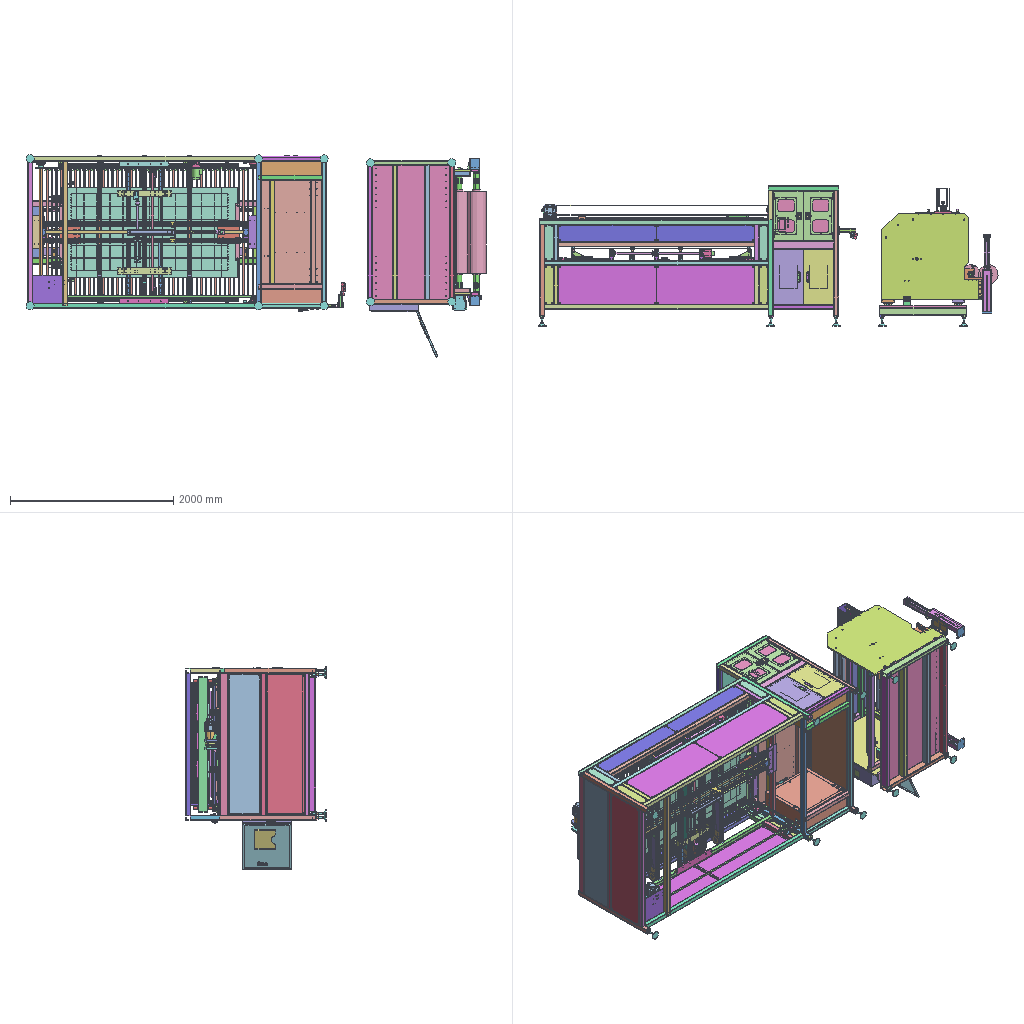Assembly | SolidWorks | 447 different items | 1108 placed | box 5632 x 1720 x 2483 mm
Parts list (item | name | quantity | parent item | size | volume | features), first 280 of 447 items:
1 | (subassembly) | x2 | in 11 | 1620 x 240 x 240 mm | 47963856 mm3 | -
2 | (subassembly) | x4 | in 1 | 35 x 74 x 74 mm | 78913 mm3 | -
3 | (subassembly) | x1 | in 11 | 170 x 962 x 160 mm | 3347225 mm3 | -
4 | (subassembly) | x1 | in 11 | 170 x 962 x 160 mm | 3347226 mm3 | -
5 | (subassembly) | x1 | in 11 | 355 x 191 x 196 mm | 4077245 mm3 | -
6 | (subassembly) | x1 | in 5 | 196 x 150 x 150 mm | 792513 mm3 | features CompositeCurve 1
7 | (subassembly) | x1 | in 11 | - | 4434874 mm3 | -
8 | (subassembly) | x2 | in 11 | 108.5 x 1345 x 60 mm | 327193 mm3 | -
9 | (subassembly) | x1 | in 11 | 130 x 80 x 80 mm | 636586 mm3 | -
10 | (subassembly) | x2 | in 58 | 70 x 30.5 x 82 mm | 109676 mm3 | -
11 | (subassembly) | x1 | - | - | 235835811 mm3 | features CompositeCurve 4
12 | (subassembly) | x1 | - | 310 x 227.812 x 145.36 mm | 532753 mm3 | -
13 | (subassembly) | x1 | - | - | - | features CompositeCurve 4, ReferencePattern 3, LocalLPattern 1
14 | (subassembly) | x1 | in 13 | - | 137447559 mm3 | features CompositeCurve 5, ReferencePattern 4, LocalLPattern 3
15 | (subassembly) | x1 | in 14 | 3660 x 1605 x 1860 mm | 102474394 mm3 | features ReferencePattern 16, LocalLPattern 3
16 | (subassembly) | x3 | in 14 | 369.222 x 614 x 49.278 mm | 1337700 mm3 | features ReferencePattern 3, CompositeCurve 1, LocalLPattern 1
17 | (subassembly) | x1 | in 14 | 369.222 x 614 x 123.704 mm | 919283 mm3 | features ReferencePattern 3, CompositeCurve 1, LocalLPattern 1
18 | (subassembly) | x1 | in 14 | 736 x 670 x 303 mm | 3762894 mm3 | features AEMSimFeature 1, MirrorCompFeat 1, ReferencePattern 1
19 | (subassembly) | x2 | in 18, 20 | 366 x 670 x 34.5 mm | 525345 mm3 | -
20 | (subassembly) | x1 | in 14 | 736 x 670 x 303 mm | 3679294 mm3 | features AEMSimFeature 1, MirrorCompFeat 1, ReferencePattern 1
21 | (subassembly) | x1 | in 13 | - | 15158359 mm3 | features ReferencePattern 23, LocalLPattern 6, CompositeCurve 3
22 | (subassembly) | x1 | in 11 | - | 105601898 mm3 | features CompositeCurve 2
23 | (subassembly) | x3 | in 21 | 45 x 115 x 115 mm | 326857 mm3 | -
24 | (subassembly) | x4 | in 21 | 45 x 50 x 50 mm | 36645 mm3 | features ReferencePattern 2, AEMSimFeature 1, MirrorCompFeat 1
25 | (subassembly) | x1 | in 13 | - | 38951088 mm3 | features ReferencePattern 10, LocalLPattern 2, AEMSimFeature 1, CompositeCurve 1
26 | (subassembly) | x1 | in 25 | 250 x 70 x 113 mm | 559339 mm3 | features AEMSimFeature 1, CompositeCurve 1
27 | (subassembly) | x1 | in 25 | 250 x 70 x 102 mm | 529348 mm3 | features AEMSimFeature 1
28 | (subassembly) | x2 | in 25 | 700 x 260 x 150.5 mm | 1942700 mm3 | features AEMSimFeature 1
29 | (subassembly) | x4 | in 28 | 40 x 40 x 85 mm | 60993 mm3 | -
30 | (subassembly) | x2 | in 25 | 666 x 259.2 x 380 mm | 1864950 mm3 | features CompositeCurve 1
31 | (subassembly) | x4 | in 30 | 58 x 169.2 x 52 mm | 267597 mm3 | -
32 | (subassembly) | x1 | in 25 | 70 x 80 x 68 mm | 209105 mm3 | features AEMSimFeature 1
33 | (subassembly) | x1 | in 22 | 837.099 x 600 x 769.432 mm | 2776594 mm3 | -
34 | (subassembly) | x1 | in 25 | 70 x 80 x 123.5 mm | 332483 mm3 | features AEMSimFeature 1
35 | (subassembly) | x1 | in 25 | 100 x 127.228 x 104 mm | 594997 mm3 | features AEMSimFeature 1, CompositeCurve 1
36 | (subassembly) | x1 | in 25 | 88 x 104 x 125 mm | 527898 mm3 | features AEMSimFeature 1
37 | (subassembly) | x1 | in 25 | 70 x 80 x 127.4 mm | 342161 mm3 | features AEMSimFeature 1
38 | (subassembly) | x1 | in 13 | - | 15629653 mm3 | features ReferencePattern 12, LocalLPattern 4, CompositeCurve 3
39 | (subassembly) | x1 | in 38 | 166.5 x 115 x 180 mm | 1052923 mm3 | features CompositeCurve 2
40 | (subassembly) | x1 | in 38 | 180 x 185 x 472 mm | 5233000 mm3 | features CompositeCurve 1
41 | (subassembly) | x1 | in 13 | - | 13271643 mm3 | features ReferencePattern 44, CompositeCurve 1, LocalLPattern 1
42 | (subassembly) | x6 | in 41 | 150 x 115.004 x 82 mm | 375409 mm3 | -
43 | (subassembly) | x1 | in 13 | 200 x 235 x 205 mm | 2926314 mm3 | -
44 | (subassembly) | x1 | in 33 | 600 x 600 x 208.5 mm | 1307519 mm3 | features LocalLPattern 1, ReferencePattern 1
45 | (subassembly) | x1 | in 13 | - | 14966347 mm3 | features ReferencePattern 9, LocalLPattern 3, CompositeCurve 2
46 | (subassembly) | x1 | in 45 | 182.5 x 100 x 174 mm | 654284 mm3 | features CompositeCurve 1
47 | (subassembly) | x1 | in 45 | 140 x 100 x 98 mm | 529951 mm3 | -
48 | (subassembly) | x1 | in 13 | - | 25836003 mm3 | -
49 | (subassembly) | x1 | in 48 | 210 x 1644 x 211.13 mm | 12241603 mm3 | features ReferencePattern 8, CompositeCurve 5, MirrorCompFeat 2
50 | (subassembly) | x1 | in 13 | - | 40703347 mm3 | features ReferencePattern 12, CompositeCurve 4, LocalLPattern 1
51 | (subassembly) | x1 | in 13 | 120 x 60 x 1710 mm | 2689604 mm3 | -
52 | (subassembly) | x1 | in 13 | 200 x 393 x 205 mm | 2855185 mm3 | -
53 | (subassembly) | x1 | in 13 | 2200 x 69.8 x 40 mm | 1056150 mm3 | features LocalLPattern 1, ReferencePattern 1
54 | (subassembly) | x8 | in 53, 57 | 22 x 67.2 x 26 mm | 3815 mm3 | features CompositeCurve 1
55 | (subassembly) | x1 | in 33 | 616.798 x 600 x 38.851 mm | 818238 mm3 | features LocalLPattern 1, ReferencePattern 1
56 | (subassembly) | x1 | in 13 | 407 x 121.237 x 1540 mm | 1039556 mm3 | -
57 | (subassembly) | x1 | in 13 | 2550 x 69.8 x 40 mm | 1229984 mm3 | features ReferencePattern 4, LocalLPattern 3
58 | (subassembly) | x2 | in 38 | 70 x 36 x 2500 mm | 1159960 mm3 | -
59 | (subassembly) | x10 | in 14, 22 | 100 x 168 x 100 mm | 203104 mm3 | -
60 | (subassembly) | x8 | in 14 | 35 x 42 x 37 mm | 5177 mm3 | -
61 | (subassembly) | x1 | in 21 | 137.5 x 90 x 275 mm | 2048853 mm3 | -
62 | (subassembly) | x1 | in 25 | 75 x 75 x 1095 mm | 1179276 mm3 | -
63 | (subassembly) | x1 | in 25 | 369 x 75 x 75 mm | 826991 mm3 | -
64 | (subassembly) | x1 | in 25 | 1100 x 2150 x 6.1 mm | 13387915 mm3 | features ReferencePattern 5, AEMSimFeature 1, LocalLPattern 1
65 | (subassembly) | x4 | in 31 | 58 x 140.2 x 52 mm | 211701 mm3 | -
66 | (subassembly) | x4 | in 11 | 60 x 60 x 1489 mm | 2237617 mm3 | -
67 | (subassembly) | x5 | in 38 | 57 x 23 x 16 mm | 13388 mm3 | -
68 | (subassembly) | x3 | in 38 | 254 x 83 x 36 mm | 461656 mm3 | -
69 | (subassembly) | x2 | in 41 | 108 x 108 x 40.2 mm | 171689 mm3 | -
70 | (subassembly) | x1 | in 45 | 130.4 x 173.65 x 80 mm | 566555 mm3 | -
71 | (subassembly) | x1 | in 46 | 49.5 x 29 x 29 mm | 22629 mm3 | -
72 | (subassembly) | x2 | in 49 | 54.62 x 52 x 58.5 mm | 87613 mm3 | -
73 | (subassembly) | x4 | in 49 | 61.5 x 41 x 96 mm | 152787 mm3 | -
74 | (subassembly) | x3 | in 50 | 116 x 77 x 84 mm | 320960 mm3 | -
75 | (subassembly) | x4 | in 50 | 60 x 45 x 400 mm | 578524 mm3 | features LocalLPattern 1, ReferencePattern 1
76 | (subassembly) | x1 | in 56 | 10 x 11.547 x 44 mm | 819.92 mm3 | -
77 | (subassembly) | x1 | in 11 | 336.706 x 259.959 x 1500 mm | 5818642 mm3 | -
78 | (subassembly) | x1 | in 11 | 527.291 x 165.21 x 90 mm | 1479501 mm3 | -
79 | (subassembly) | x4 | in 22 | 100 x 48 x 360 mm | 575184 mm3 | -
80 | (subassembly) | x2 | in 55 | 26.164 x 73 x 27.149 mm | 6971 mm3 | -
81 | (subassembly) | x2 | in 3, 4 | 792.217 x 75 x 75 mm | 831680 mm3 | -
82 | (subassembly) | x1 | in 5 | 167 x 205 x 191 mm | 3156838 mm3 | -
83 | (subassembly) | x4 | in 8 | 61.5 x 44 x 50 mm | 72597 mm3 | -
84 | (subassembly) | x2 | in 7 | 96.283 x 62 x 71.5 mm | 157551 mm3 | -
85 | (subassembly) | x2 | in 18, 20 | 366 x 670 x 34.5 mm | 525345 mm3 | -
86 | (subassembly) | x2 | in 77 | 60 x 60 x 1352 mm | 1988241 mm3 | -
87 | - | x1 | in 11 | 26.731 x 568.268 x 1527 mm | 1309231 mm3 | features ICE 3, EdgeFlange 2, MirrorPattern 2, FlatPattern 1, HoleWzd 1, LPattern 1, SMBaseFlange 1, SheetMetal 1
88 | - | x4 | in 21 | 550 x 145 x 6 mm | 278339 mm3 | features Fillet 4, HoleWzd 3, MirrorPattern 2, EdgeFlange 1, FlatPattern 1, ICE 1, SMBaseFlange 1, SheetMetal 1
89 | - | x1 | in 21 | 45 x 145 x 1860 mm | 2040055 mm3 | features ICE 10, Fillet 8, MirrorPattern 2, Extrusion 1, LPattern 1
90 | - | x4 | in 23, 39 | 37 x 115 x 115 mm | 284316 mm3 | features ICE 5, Fillet 2, CirPattern 1, Extrusion 1, MirrorPattern 1, RevCut 1
91 | - | x3 | in 23 | 45 x 20 x 20 mm | 12570 mm3 | features MirrorPattern 2, Chamfer 1, Extrusion 1, HoleWzd 1, RevCut 1
92 | - | x4 | in 24 | 37 x 50 x 50 mm | 19824 mm3 | features ICE 5, Fillet 2, MirrorPattern 2, CirPattern 1, Extrusion 1, RevCut 1
93 | - | x4 | in 24 | 15 x 15 x 45 mm | 6384 mm3 | features MirrorPattern 2, Chamfer 1, Extrusion 1, HoleWzd 1, RevCut 1
94 | - | x1 | in 25 | 2720 x 1720 x 50 mm | 8199509 mm3 | features WeldCornerFeat 6, WeldMemberFeat 3, 3DProfileFeature 1, HoleWzd 1, WeldmentFeature 1
95 | - | x8 | in 25 | 23 x 22 x 20 mm | 8934 mm3 | features Chamfer 1, Extrusion 1, HoleWzd 1
96 | - | x1 | in 25 | 76 x 140 x 60 mm | 135317 mm3 | features ICE 2, 3DProfileFeature 1, HoleWzd 1, WeldMemberFeat 1, WeldmentFeature 1
97 | - | x2 | in 25 | 60 x 146 x 55 mm | 90878 mm3 | features HoleWzd 2, ICE 2, 3DProfileFeature 1, Fillet 1, WeldMemberFeat 1, WeldmentFeature 1
98 | - | x2 | in 11 | 86 x 50 x 50 mm | 32616 mm3 | features Chamfer 1, Extrusion 1, ICE 1, Revolution 1
99 | - | x1 | in 25 | 60 x 30 x 90 mm | 136711 mm3 | features HoleWzd 2, Chamfer 1, Extrusion 1
100 | - | x2 | in 25 | 320 x 80 x 12 mm | 298012 mm3 | features HoleWzd 3, Chamfer 1, Extrusion 1
101 | - | x1 | in 25 | 10 x 138 x 100 mm | 115642 mm3 | features HoleWzd 2, Chamfer 1, CirPattern 1, Extrusion 1, ICE 1
102 | - | x2 | in 25 | 12 x 80 x 128 mm | 113628 mm3 | features HoleWzd 2, Chamfer 1, Extrusion 1
103 | - | x1 | in 25 | 60 x 50 x 90 mm | 182634 mm3 | features Chamfer 2, HoleWzd 2, Extrusion 1, ICE 1
104 | - | x1 | in 25 | 50 x 25 x 25 mm | 16197 mm3 | features Chamfer 1, Extrusion 1, HoleWzd 1, ICE 1
105 | - | x1 | in 25 | 16 x 16 x 350 mm | 70372 mm3 | features Extrusion 1
106 | - | x1 | in 25 | 12.4 x 70 x 80 mm | 67492 mm3 | features HoleWzd 2, Extrusion 1
107 | - | x1 | in 25 | 70 x 80 x 12 mm | 61436 mm3 | features Chamfer 1, Extrusion 1, HoleWzd 1, ICE 1, LPattern 1
108 | - | x2 | in 26, 27 | 250 x 70 x 12 mm | 205147 mm3 | features HoleWzd 3, Chamfer 1, Extrusion 1
109 | - | x1 | in 11 | 50 x 58 x 120 mm | 53105 mm3 | features EdgeFlange 2, HoleWzd 2, Chamfer 1, CirPattern 1, FlatPattern 1, ICE 1, SMBaseFlange 1, SheetMetal 1
110 | - | x2 | in 26 | 70 x 101 x 12 mm | 76361 mm3 | features ICE 3, Chamfer 1, Extrusion 1, HoleWzd 1
111 | - | x2 | in 26, 45 | - | - | features RefSurface 1
112 | - | x1 | in 26 | 20 x 20 x 100 mm | 29039 mm3 | features ICE 3, Chamfer 1, Extrusion 1, MirrorPattern 1
113 | - | x2 | in 26, 27 | 80 x 70 x 10 mm | 55201 mm3 | features HoleWzd 2, Extrusion 1
114 | - | x2 | in 27 | 70 x 90 x 12 mm | 66580 mm3 | features ICE 2, Cut 1, Extrusion 1, HoleWzd 1
115 | - | x2 | in 27, 45 | 37 x 67 x 67 mm | 77744 mm3 | features ICE 3, BaseBody 2
116 | - | x1 | in 27 | 17 x 17 x 104 mm | 22466 mm3 | features Chamfer 1, Extrusion 1, HoleWzd 1, ICE 1, MirrorPattern 1
117 | - | x2 | in 27 | 22 x 22 x 21.5 mm | 3204 mm3 | features Chamfer 1, Extrusion 1
118 | - | x2 | in 28 | 700 x 40 x 15 mm | 415141 mm3 | features HoleWzd 2, Chamfer 1, Extrusion 1
119 | - | x4 | in 29 | 40 x 40 x 43 mm | 42314 mm3 | features ICE 3, Chamfer 1, Extrusion 1
120 | - | x1 | in 11 | 43 x 10 x 10 mm | 2787 mm3 | features ICE 3, Extrusion 1
121 | - | x2 | in 28 | 280 x 260 x 15 mm | 1077641 mm3 | features HoleWzd 4, Chamfer 1, Extrusion 1
122 | - | x2 | in 28 | 280 x 60 x 12 mm | 196575 mm3 | features HoleWzd 3, Extrusion 1
123 | - | x4 | in 28 | 140 x 60 x 12 mm | 65678 mm3 | features HoleWzd 3, Extrusion 1
124 | - | x4 | in 30 | 23 x 22 x 20 mm | 8802 mm3 | features Chamfer 1, Extrusion 1, HoleWzd 1
125 | - | x4 | in 31 | 50 x 27 x 50 mm | 32903 mm3 | features Chamfer 2, ICE 2, Extrusion 1, RevCut 1
126 | - | x4 | in 31 | 25 x 20 x 25 mm | 7104 mm3 | features Chamfer 2, ICE 2, Extrusion 1
127 | - | x4 | in 31 | 25 x 3 x 25 mm | 1262 mm3 | features Chamfer 1, Extrusion 1, ICE 1
128 | - | x2 | in 30 | 90 x 80 x 666 mm | 761508 mm3 | features HoleWzd 4, EdgeFlange 2, Chamfer 1, FlatPattern 1, MirrorPattern 1, SMBaseFlange 1, SheetMetal 1
129 | - | x1 | in 32 | 70 x 80 x 12 mm | 63058 mm3 | features HoleWzd 2, Extrusion 1
130 | - | x2 | in 32 | 80 x 39 x 14 mm | 42305 mm3 | features HoleWzd 2, Extrusion 1
131 | - | x1 | in 11 | 51 x 40 x 90 mm | 135826 mm3 | features HoleWzd 2, Extrusion 1
132 | - | x1 | in 32 | 70 x 80 x 12 mm | 61436 mm3 | features Chamfer 1, Extrusion 1, HoleWzd 1, ICE 1, LPattern 1
133 | - | x1 | in 34 | 70 x 80 x 12 mm | 59166 mm3 | features HoleWzd 2, Cut 1, Extrusion 1, LPattern 1
134 | - | x2 | in 34 | 80 x 94.5 x 14 mm | 104465 mm3 | features HoleWzd 2, Extrusion 1
135 | - | x1 | in 34 | 70 x 80 x 12 mm | 64386 mm3 | features HoleWzd 2, Chamfer 1, Extrusion 1, ICE 1, LPattern 1
136 | - | x2 | in 35 | 80 x 125 x 14 mm | 129543 mm3 | features ICE 3, Chamfer 1, Extrusion 1, HoleWzd 1
137 | - | x1 | in 35 | 20 x 20 x 100 mm | 29039 mm3 | features ICE 3, Chamfer 1, Extrusion 1, MirrorPattern 1
138 | - | x2 | in 35, 36 | 60 x 80 x 10 mm | 47201 mm3 | features HoleWzd 2, Extrusion 1
139 | - | x1 | in 35 | 37.864 x 104 x 104 mm | 230318 mm3 | features ICE 2, BaseBody 1
140 | - | x2 | in 36 | 81 x 125 x 14 mm | 129784 mm3 | features ICE 2, Cut 1, Extrusion 1, HoleWzd 1
141 | - | x1 | in 36 | 17 x 17 x 84 mm | 17880 mm3 | features Chamfer 1, Extrusion 1, HoleWzd 1, ICE 1, MirrorPattern 1, RevCut 1
142 | - | x1 | in 22 | 132 x 1060 x 1760 mm | 42498587 mm3 | features MirrorPattern 5, HoleWzd 3, ICE 2, LPattern 1, WeldMemberFeat 1, WeldmentFeature 1
143 | - | x1 | in 36 | 37.864 x 104 x 104 mm | 203249 mm3 | features ICE 3, BaseBody 1
144 | - | x1 | in 37 | 70 x 80 x 12 mm | 63058 mm3 | features HoleWzd 2, Extrusion 1
145 | - | x2 | in 37 | 80 x 98.4 x 14 mm | 108833 mm3 | features HoleWzd 2, Extrusion 1
146 | - | x1 | in 37 | 70 x 80 x 12 mm | 61436 mm3 | features Chamfer 1, Extrusion 1, HoleWzd 1, ICE 1, LPattern 1
147 | - | x1 | in 38 | 900 x 16 x 80 mm | 1104727 mm3 | features HoleWzd 4, Extrusion 1, ICE 1, LPattern 1, MirrorPattern 1
148 | - | x1 | in 38 | 12 x 50 x 100 mm | 56676 mm3 | features Chamfer 1, Extrusion 1, HoleWzd 1
149 | - | x3 | in 38 | 20 x 200 x 80 mm | 318272 mm3 | features HoleWzd 2, Extrusion 1
150 | - | x1 | in 38 | 40 x 1200 x 20 mm | 255420 mm3 | features HoleWzd 1, LPattern 1, WeldMemberFeat 1, WeldmentFeature 1
151 | - | x5 | in 38 | 70 x 20 x 55 mm | 50750 mm3 | features HoleWzd 3, ICE 3, Chamfer 1, Extrusion 1, Fillet 1
152 | - | x1 | in 38 | 900 x 16 x 120 mm | 1714971 mm3 | features HoleWzd 2, Extrusion 1, LPattern 1, MirrorPattern 1
153 | - | x1 | in 22 | 1607 x 1230 x 1105 mm | 56719734 mm3 | features Chamfer 12, HoleWzd 12, ICE 6, WeldCornerFeat 4, LPattern 3, WeldMemberFeat 3, MirrorPattern 2, EndCap 1, WeldmentFeature 1
154 | - | x3 | in 38 | 12 x 80 x 160 mm | 149467 mm3 | features HoleWzd 2, Extrusion 1
155 | - | x1 | in 38 | 30 x 31 x 20 mm | 1948 mm3 | features EdgeFlange 1, FlatPattern 1, HoleWzd 1, ICE 1, SMBaseFlange 1, SheetMetal 1
156 | - | x2 | in 39 | 20 x 140 x 100 mm | 250918 mm3 | features HoleWzd 4, Extrusion 1, ICE 1
157 | - | x2 | in 39, 47 | 20 x 98 x 20 mm | 28115 mm3 | features Extrusion 1, HoleWzd 1, ICE 1, RevCut 1
158 | - | x1 | in 39 | 12 x 100 x 180 mm | 209434 mm3 | features HoleWzd 2, Chamfer 1, Extrusion 1
159 | - | x1 | in 40 | 16 x 160 x 350 mm | 884211 mm3 | features HoleWzd 2, Chamfer 1, Extrusion 1
160 | - | x1 | in 40 | 120 x 164 x 160 mm | 840772 mm3 | features ICE 6, HoleWzd 2, Chamfer 1, CirPattern 1, Extrusion 1, LPattern 1
161 | - | x1 | in 40 | 80 x 164 x 160 mm | 773961 mm3 | features ICE 5, Chamfer 1, Extrusion 1, HoleWzd 1
162 | - | x1 | in 40 | 110 x 130 x 130 mm | 397352 mm3 | features ICE 5, CirPattern 2, HoleWzd 2, Chamfer 1, Extrusion 1
163 | - | x1 | in 40 | 37 x 115 x 115 mm | 319637 mm3 | features ICE 8, CirPattern 2, Fillet 2, MirrorPattern 2, Extrusion 1, HoleWzd 1, RevCut 1
164 | - | x2 | in 22 | 20 x 125 x 223 mm | 246915 mm3 | features Chamfer 2, HoleWzd 2, ICE 2, Extrusion 1, Fillet 1, LPattern 1
165 | - | x1 | in 40 | 140 x 25 x 25 mm | 55450 mm3 | features ICE 3, Extrusion 1, RevCut 1
166 | - | x2 | in 41 | 30.001 x 114.527 x 115.015 mm | 100872 mm3 | features ICE 4, BaseBody 1, Fillet 1, RevCut 1
167 | - | x1 | in 41 | 1705 x 40 x 40 mm | 2098690 mm3 | features ICE 3, RevCut 2, Extrusion 1, LPattern 1
168 | - | x1 | in 41 | 30.001 x 163.166 x 163.486 mm | 245205 mm3 | features ICE 3, BaseBody 1, CirPattern 1, HoleWzd 1
169 | - | x45 | in 41 | 20 x 1546 x 10 mm | 86388 mm3 | features Extrusion 1, HoleWzd 1, WeldmentFeature 1
170 | - | x1 | in 41 | 10 x 16 x 65 mm | 2116 mm3 | features EdgeFlange 1, FlatPattern 1, HoleWzd 1, ICE 1, SMBaseFlange 1, SheetMetal 1
171 | - | x6 | in 42 | 6 x 35 x 35 mm | 5391 mm3 | features Extrusion 1
172 | - | x6 | in 42 | 100 x 100 x 66 mm | 144315 mm3 | features HoleWzd 2, ICE 2, CirPattern 1, Extrusion 1, Fillet 1
173 | - | x6 | in 42 | 10 x 100 x 150 mm | 126323 mm3 | features Chamfer 1, Extrusion 1, HoleWzd 1, ICE 1
174 | - | x6 | in 42 | 40.001 x 114.527 x 115.015 mm | 88527 mm3 | features ICE 6, BaseBody 1, Fillet 1, RevCut 1
175 | - | x1 | in 44 | 600 x 600 x 208.5 mm | 1302353 mm3 | features ICE 4, EdgeFlange 3, FlatPattern 1, HoleWzd 1, SMBaseFlange 1, SheetMetal 1
176 | - | x2 | in 43, 52 | 120 x 194 x 200 mm | 863954 mm3 | features ICE 7, Chamfer 1, CirPattern 1, Extrusion 1, HoleWzd 1
177 | - | x1 | in 43 | 30.001 x 114.527 x 115.015 mm | 126258 mm3 | features BaseBody 1, Chamfer 1, CirPattern 1, HoleWzd 1
178 | - | x1 | in 45 | 20 x 136 x 1840 mm | 4958995 mm3 | features HoleWzd 2, Extrusion 1, LPattern 1
179 | - | x4 | in 45 | 20 x 100 x 136 mm | 267548 mm3 | features HoleWzd 2, Extrusion 1
180 | - | x1 | in 45 | 20 x 140 x 100 mm | 253738 mm3 | features HoleWzd 2, ICE 2, Extrusion 1
181 | - | x1 | in 45 | 20 x 140 x 100 mm | 250976 mm3 | features HoleWzd 3, ICE 2, Extrusion 1
182 | - | x1 | in 45 | 150 x 20 x 20 mm | 38325 mm3 | features ICE 3, Extrusion 1, RevCut 1
183 | - | x1 | in 45 | 90 x 85 x 85 mm | 146439 mm3 | features ICE 5, CirPattern 2, HoleWzd 2, Extrusion 1
184 | - | x1 | in 45 | 14 x 120 x 1840 mm | 3046855 mm3 | features HoleWzd 5, ICE 2, LPattern 2, Extrusion 1
185 | - | x1 | in 45 | 20 x 100 x 120 mm | 234911 mm3 | features Extrusion 1, HoleWzd 1
186 | - | x2 | in 44 | 20 x 36 x 19.5 mm | 2583 mm3 | features EdgeFlange 1, FlatPattern 1, HoleWzd 1, SMBaseFlange 1, SheetMetal 1
187 | - | x1 | in 45 | 20 x 100 x 120 mm | 213797 mm3 | features HoleWzd 2, Extrusion 1, ICE 1
188 | - | x2 | in 45 | 10 x 100 x 98 mm | 95455 mm3 | features Extrusion 1, HoleWzd 1
189 | - | x1 | in 45 | 40 x 1650 x 40 mm | 782541 mm3 | features HoleWzd 1, LPattern 1, WeldMemberFeat 1, WeldmentFeature 1
190 | - | x4 | in 45 | 30 x 30 x 5 mm | 4066 mm3 | features Extrusion 1, HoleWzd 1
191 | - | x1 | in 46 | 50 x 45 x 68 mm | 67005 mm3 | features HoleWzd 4, Cut 2, Extrusion 1, ICE 1
192 | - | x1 | in 46 | 100 x 65 x 15 mm | 94078 mm3 | features HoleWzd 4, Extrusion 1
193 | - | x1 | in 46 | 60 x 25 x 16 mm | 6607 mm3 | features ICE 5, Fillet 2, MirrorPattern 2, Chamfer 1, Extrusion 1, HoleWzd 1
194 | - | x1 | in 46 | 20 x 28 x 27 mm | 4092 mm3 | features ICE 3, Chamfer 2, HoleWzd 2, Extrusion 1
195 | - | x1 | in 46 | 32 x 32 x 68 mm | 22395 mm3 | features ICE 4, RevCut 2, Chamfer 1, Extrusion 1
196 | - | x1 | in 46 | 21 x 21 x 60 mm | 13278 mm3 | features ICE 4, Chamfer 1, Extrusion 1, HoleWzd 1
197 | - | x2 | in 78 | 47.2 x 12 x 12 mm | 5259 mm3 | features BaseBody 1
198 | - | x1 | in 33 | 500 x 500 x 2 mm | 469692 mm3 | features Extrusion 1, HoleWzd 1, ICE 1
199 | - | x1 | in 46 | 22 x 22 x 25 mm | 3110 mm3 | features Chamfer 1, Extrusion 1
200 | - | x1 | in 46 | 24 x 24 x 10 mm | 4256 mm3 | features Chamfer 1, Extrusion 1, ICE 1
201 | - | x1 | in 46 | 92 x 92 x 3 mm | 18153 mm3 | features Chamfer 1, Extrusion 1, ICE 1
202 | - | x2 | in 46 | 24 x 43 x 10 mm | 6079 mm3 | features HoleWzd 2, Cut 1, Extrusion 1, Fillet 1
203 | - | x1 | in 46 | 100 x 50 x 15 mm | 66421 mm3 | features Chamfer 1, Extrusion 1, HoleWzd 1, ICE 1
204 | - | x1 | in 46 | 53.5 x 58 x 30 mm | 4665 mm3 | features ExtruThin 1, Fillet 1, ICE 1
205 | - | x1 | in 46 | 50 x 45 x 35 mm | 39850 mm3 | features HoleWzd 3, Chamfer 1, Extrusion 1, ICE 1
206 | - | x1 | in 46 | 8 x 32 x 40 mm | 7835 mm3 | features HoleWzd 2, Extrusion 1, ICE 1
207 | - | x1 | in 46 | 10 x 47 x 100 mm | 42728 mm3 | features HoleWzd 3, Extrusion 1
208 | - | x1 | in 46 | 10 x 70 x 100 mm | 64355 mm3 | features HoleWzd 3, Extrusion 1
209 | - | x1 | in 55 | 600 x 600 x 22 mm | 660192 mm3 | features EdgeFlange 2, ICE 2, FlatPattern 1, SMBaseFlange 1, SheetMetal 1
210 | - | x1 | in 46 | 10 x 100 x 85 mm | 82523 mm3 | features HoleWzd 2, Extrusion 1
211 | - | x2 | in 47 | 20 x 140 x 100 mm | 250918 mm3 | features HoleWzd 4, Extrusion 1, ICE 1
212 | - | x2 | in 48 | 272 x 130 x 210 mm | 2006096 mm3 | features ICE 5, HoleWzd 3, Chamfer 1, Extrusion 1, Fillet 1
213 | - | x1 | in 48 | 133.771 x 133.771 x 26 mm | 282633 mm3 | features ICE 2, CirPattern 1, Cut 1, RefAxis 1, Revolution 1
214 | - | x1 | in 48 | 96 x 96 x 1659 mm | 9258344 mm3 | features ICE 6, Chamfer 1, Cut 1, Extrusion 1, LPattern 1, RevCut 1
215 | - | x4 | in 49 | 20 x 20 x 130 mm | 39341 mm3 | features HoleWzd 2, Chamfer 1, Extrusion 1
216 | - | x1 | in 49 | 160 x 100 x 12 mm | 181929 mm3 | features HoleWzd 4, Chamfer 1, Extrusion 1
217 | - | x2 | in 49 | 210 x 80 x 12 mm | 144293 mm3 | features HoleWzd 3, Chamfer 1, Cut 1, Extrusion 1, ICE 1
218 | - | x2 | in 49 | 46 x 30 x 12 mm | 11866 mm3 | features HoleWzd 2, Chamfer 1, Extrusion 1, ICE 1
219 | - | x1 | in 49 | 140 x 40 x 16 mm | 80881 mm3 | features HoleWzd 2, Chamfer 1, Extrusion 1
220 | - | x1 | in 55 | 250 x 250 x 30 mm | 118526 mm3 | features EdgeFlange 1, Fillet 1, FlatPattern 1, ICE 1, SMBaseFlange 1, SheetMetal 1
221 | - | x1 | in 49 | 96 x 96 x 1500 mm | 10059847 mm3 | features ICE 4, Helix 2, Chamfer 1, CirPattern 1, Extrusion 1, MirrorPattern 1, SweepCut 1
222 | - | x2 | in 49 | 35 x 35 x 3 mm | 1869 mm3 | features Chamfer 1, Extrusion 1
223 | - | x2 | in 49 | 80 x 70 x 35 mm | 87735 mm3 | features ICE 5, Chamfer 1, Extrusion 1, HoleWzd 1
224 | - | x2 | in 49 | 25 x 20 x 20 mm | 3580 mm3 | features Extrusion 1, HoleWzd 1, ICE 1
225 | - | x1 | in 50 | 50 x 150 x 1660 mm | 10088641 mm3 | features HoleWzd 5, MirrorPattern 4, Chamfer 1, Extrusion 1, ICE 1, LPattern 1
226 | - | x1 | in 50 | 120 x 120 x 1660 mm | 15602206 mm3 | features ICE 2, Chamfer 1, Extrusion 1
227 | - | x2 | in 50 | 100 x 100 x 450 mm | 742625 mm3 | features Chamfer 1, CirPattern 1, Extrusion 1, HoleWzd 1, ICE 1
228 | - | x3 | in 50 | 20 x 120 x 200 mm | 471931 mm3 | features Chamfer 1, Extrusion 1, HoleWzd 1
229 | - | x3 | in 50 | 20 x 120 x 200 mm | 467167 mm3 | features HoleWzd 2, Chamfer 1, Extrusion 1
230 | - | x3 | in 50 | 80 x 100 x 100 mm | 263043 mm3 | features HoleWzd 3, ICE 2, Chamfer 1, CirPattern 1, Extrusion 1, Fillet 1
231 | - | x4 | in 66 | 25 x 25 x 1487 mm | 729820 mm3 | features ICE 3, Extrusion 1, RevCut 1
232 | - | x3 | in 50 | 20 x 80 x 100 mm | 149224 mm3 | features HoleWzd 2, Chamfer 1, Extrusion 1
233 | - | x3 | in 50 | 30 x 30 x 100 mm | 70744 mm3 | features HoleWzd 2, Chamfer 1, Extrusion 1, ICE 1
234 | - | x2 | in 50 | 15 x 150 x 400 mm | 888167 mm3 | features Extrusion 1, HoleWzd 1
235 | - | x1 | in 50 | 15 x 150 x 150 mm | 329611 mm3 | features Extrusion 1, HoleWzd 1
236 | - | x2 | in 50 | 0.5 x 25 x 70 mm | 816.894 mm3 | features Extrusion 1, HoleWzd 1, ICE 1
237 | - | x1 | in 50 | 15 x 15 x 72 mm | 14194 mm3 | features Extrusion 1, HoleWzd 1
238 | - | x2 | in 50 | 30 x 450 x 150 mm | 1472324 mm3 | features HoleWzd 3, ICE 2, LPattern 2, Extrusion 1
239 | - | x2 | in 50 | 45 x 45 x 50 mm | 47153 mm3 | features Chamfer 2, HoleWzd 2, Extrusion 1, ICE 1
240 | - | x2 | in 50 | 950 x 70 x 70 mm | 294808 mm3 | features ICE 3, Chamfer 1, Extrusion 1, Fillet 1
241 | - | x2 | in 50 | 47 x 25 x 90 mm | 53619 mm3 | features Chamfer 2, HoleWzd 2, Extrusion 1, ICE 1
242 | - | x1 | in 77 | 30 x 30 x 1500 mm | 1054135 mm3 | features Extrusion 1, HoleWzd 1, ICE 1, LPattern 1, RevCut 1
243 | - | x1 | in 50 | 49.96 x 24 x 80 mm | 59562 mm3 | features Chamfer 1, Extrusion 1, HoleWzd 1, ICE 1
244 | - | x1 | in 50 | 49.96 x 24 x 80 mm | 61914 mm3 | features Chamfer 1, Extrusion 1, HoleWzd 1
245 | - | x1 | in 51 | 25 x 25 x 1600 mm | 783785 mm3 | features Chamfer 1, Extrusion 1, HoleWzd 1, MirrorPattern 1, RevCut 1
246 | - | x5 | in 51, 66 | 60 x 60 x 1480 mm | 1496944 mm3 | features ICE 3, Chamfer 1, Extrusion 1
247 | - | x2 | in 51 | 109 x 90 x 50 mm | 199011 mm3 | features ICE 5, HoleWzd 3, Chamfer 1, Extrusion 1
248 | - | x1 | in 52 | 55 x 55 x 26 mm | 25939 mm3 | features CirPattern 2, Cut 2, ICE 2, RefAxis 1, RevCut 1, Revolution 1
249 | - | x2 | in 13, 53 | 40 x 2200 x 40 mm | 1044704 mm3 | features WeldMemberFeat 1, WeldmentFeature 1
250 | - | x8 | in 54 | 22 x 17 x 26 mm | 1786 mm3 | features Fillet 3, ExtruThin 1, HoleWzd 1, ICE 1
251 | - | x1 | in 56 | 1540 x 18.5 x 407 mm | 949433 mm3 | features ICE 4, HoleWzd 2, LPattern 2, EdgeFlange 1, FlatPattern 1, SMBaseFlange 1, SheetMetal 1
252 | - | x4 | in 56 | 117 x 15 x 15 mm | 20237 mm3 | features HoleWzd 2, Chamfer 1, Extrusion 1
253 | - | x2 | in 77 | 60 x 345 x 50 mm | 297279 mm3 | features ICE 2, Extrusion 1, HoleWzd 1
254 | - | x1 | in 56 | 43 x 32 x 13 mm | 8354 mm3 | features ICE 2, Extrusion 1, Fillet 1, HoleWzd 1
255 | - | x1 | in 57 | 40 x 2550 x 40 mm | 1210907 mm3 | features WeldMemberFeat 1, WeldmentFeature 1
256 | - | x1 | in 82 | 23.8 x 23.8 x 191 mm | 54008 mm3 | features BaseBody 1
257 | - | x1 | in 82 | 42 x 42 x 167 mm | 107574 mm3 | features ICE 3, BaseBody 1
258 | - | x1 | in 82 | 47.6 x 47.6 x 120 mm | 130851 mm3 | features BaseBody 1
259 | - | x1 | in 13 | 18.8 x 183.6 x 389.75 mm | 274842 mm3 | features ExtruThin 1
260 | - | x1 | in 13 | 1895 x 190 x 79 mm | 7147042 mm3 | features HoleWzd 2, Extrusion 1
261 | - | x1 | in 14 | 271 x 213 x 36.36 mm | 1748728 mm3 | features Fillet 2, ICE 2, Extrusion 1
262 | - | x1 | in 14 | 62 x 130 x 130 mm | 835738 mm3 | features ICE 2, Extrusion 1
263 | - | x4 | in 16, 17 | 60 x 94 x 17 mm | 35696 mm3 | features BaseBody 1
264 | - | x2 | in 86 | 25 x 25 x 1352 mm | 663661 mm3 | features Extrusion 1
265 | - | x8 | in 16, 17 | - | - | features RefSurface 3
266 | - | x8 | in 16, 17 | 22.778 x 15.778 x 36 mm | 3424 mm3 | features EdgeFlange 2, FlatPattern 1, Hem 1, HoleWzd 1, SMBaseFlange 1, SheetMetal 1
267 | - | x8 | in 16, 17 | 20 x 36 x 19.5 mm | 2583 mm3 | features EdgeFlange 1, FlatPattern 1, HoleWzd 1, SMBaseFlange 1, SheetMetal 1
268 | - | x1 | in 17 | 66 x 102.704 x 66 mm | 215531 mm3 | features BaseBody 1
269 | - | x1 | in 17 | 42.5 x 70.184 x 39.6 mm | 56973 mm3 | features Boss 6, Cut 2, Extrusion 1, Revolution 1
270 | - | x2 | in 17 | 42 x 32 x 92.5 mm | 74661 mm3 | features ICE 36, MirrorPattern 8, ConnectionPoint 4, Fillet 4, PLine 2, SmartComponentFeature 1
271 | - | x2 | in 19 | 124 x 67 x 29 mm | 25577 mm3 | features ICE 3, Extrusion 1
272 | - | x3 | in 21 | 30 x 121.59 x 1872 mm | 524754 mm3 | features ExtruThin 1
273 | - | x2 | in 21 | 95 x 24.5 x 64 mm | 45810 mm3 | features ICE 7, Extrusion 1, MirrorPattern 1
274 | - | x4 | in 25 | 23 x 22 x 610 mm | 258583 mm3 | features ICE 4, BaseBody 1, HoleWzd 1, LPattern 1
275 | - | x2 | in 86 | 60 x 60 x 1300 mm | 1313726 mm3 | features ICE 3, Chamfer 1, Extrusion 1
276 | - | x8 | in 25, 30 | 70 x 30.5 x 84 mm | 110295 mm3 | features BaseBody 1
277 | - | x2 | in 25 | 44.5 x 44.5 x 90 mm | 81124 mm3 | features BaseBody 1
278 | - | x1 | in 25 | 2564 x 70.66 x 30 mm | 701169 mm3 | features ExtruThin 1
279 | - | x1 | in 25 | 30 x 102.5 x 1599 mm | 445594 mm3 | features ExtruThin 1
280 | - | x4 | in 30 | 340 x 22 x 23 mm | 165043 mm3 | features Extrusion 1, HoleWzd 1, LPattern 1
Mates (type | each side: item.copy, entity, surface, feature), first 304 of 1303 lines:
In the top assembly
Coincident | 406.1 face plane Revolve 1 | 406.2 face plane Revolve 1
Parallel | 424.1 face plane Square Tube 60 X 60 X 5.0(1) | 142.1 face plane Rectangular Tube 100 X 60 X 5.0(1)
Width | 142.1 face plane Rectangular Tube 100 X 60 X 5.0(1) | 142.1 face plane Rectangular Tube 100 X 60 X 5.0(1) | 424.1 face plane Square Tube 60 X 60 X 5.0(1) | 424.1 face plane Square Tube 60 X 60 X 5.0(1)
Coincident | 424.1 face plane Square Tube 60 X 60 X 5.0(1) | 400.1 face plane Boss-Extrude 1
Coincident | 424.1 face plane Rectangular Tube 100 X 60 X 5.0(3) | 400.1 face plane Boss-Extrude 1
Concentric | 424.1 face cylinder M8 Tapped Hole 8 | 400.1 face cylinder Ø9.0 (9) DiameterHole 1
In subassembly 11
Concentric | 87.1 edge | 388.1 face cylinder Boss-Extrude 2
Concentric | 87.1 face cylinder Cut-Extrude 1 | 388.2 face cylinder Boss-Extrude 2
Coincident | 98.1 face plane Boss-Extrude 1 | 98.2 face plane Boss-Extrude 1
Coincident | 390.1 face plane Boss-Extrude 1 | 391.1 face plane Boss-Extrude 1
Concentric | 390.1 face cylinder Drill Hole Size (% per) Socket Head Cap Screw Type 1 | 391.1 face cylinder M10 Tapped Hole 1 | 2 times
Coincident | 242.1 face plane Boss-Extrude 1 | 120.1 face plane Boss-Extrude 2
Concentric | 242.1 face cylinder M8 Tapped Hole 1 | 120.1 face cylinder Boss-Extrude 2
Concentric | 109.1 face cylinder Cut-Extrude 1 | 299.1 face cylinder Boss-Extrude 2
Coincident | 109.1 face plane Base-Flange 1 | 299.1 face plane Boss-Extrude 1
Concentric | 299.1 face cylinder Boss-Extrude 2 | 300.1 face cylinder Import 1
Concentric | 120.1 face cylinder Boss-Extrude 2 | 300.1 face cylinder Import 1
Tangent | 331.1 face plane Boss-Extrude 1 | 309.1 face cylinder Revolve 1
Coincident | 331.1 face plane Boss-Extrude 1 | 309.1 face plane Revolve 1
Concentric | 286.1 face cylinder Boss-Extrude 6 | 352.1 face cylinder Bore
Coincident | 286.1 face plane Boss-Extrude 2 | 352.1 face plane Base-Revolve
Concentric | 142.2 edge | 370.1 face cylinder Import 1
Coincident | 142.2 face plane Boss-Extrude 1 | 131.1 face plane Boss-Extrude 1
Coincident | 370.1 face plane Import 1 | 131.1 face plane Boss-Extrude 1 | 3 times
Concentric | 153.1 face cylinder Ø16.0 (16) DiameterHole 1 | 246.1 face cylinder Boss-Extrude 1
Concentric | 153.1 face cylinder Ø16.0 (16) DiameterHole 1 | 246.2 face cylinder Boss-Extrude 1
Concentric | 153.1 face cylinder Cut-Extrude 1 | 242.1 face cylinder Boss-Extrude 1
Concentric | 153.1 edge | 231.1 face cylinder Boss-Extrude 1
Concentric | 153.1 face cylinder Ø16.0 (16) DiameterHole 1 | 246.3 face cylinder Boss-Extrude 1
Coincident | 153.1 face plane Boss-Extrude 3 | 342.1 face plane Edge-Flange 1
Coincident | 153.1 face plane Boss-Extrude 5 | 380.1 face plane Boss-Extrude 1
Parallel | 153.1 face plane Boss-Extrude 5 | 386.1 face plane Edge-Flange 1
Coincident | 153.1 face plane Boss-Extrude 2 | 231.2 face plane Cut-Extrude 3
Coincident | 153.1 face plane Boss-Extrude 3 | 231.3 face plane Cut-Extrude 2
Coincident | 153.1 face plane Boss-Extrude 3 | 231.4 face plane Cut-Extrude 2
Coincident | 153.1 face plane Boss-Extrude 3 | 231.1 face plane Cut-Extrude 2
Concentric | 153.1 face cylinder M10 Tapped Hole 1 | 380.1 face cylinder Ø12.5 (12.5) DiameterHole 1 | 2 times
Coincident | 153.1 face plane Rectangular Tube 60X30X4(1) | 387.1 face plane Boss-Extrude 1
Concentric | 153.1 face cylinder M6 Tapped Hole 1 | 387.1 face cylinder Ø7.0 (7) DiameterHole 1 | 2 times
Coincident | 153.1 face plane Rectangular Tube 60X30X4(1) | 387.2 face plane Boss-Extrude 1
Concentric | 153.1 face cylinder M6 Tapped Hole 1 | 387.2 face cylinder Ø7.0 (7) DiameterHole 1 | 2 times
Coincident | 153.1 face plane Rectangular Tube 60X30X4(1) | 87.1 face plane Base-Flange 1
Concentric | 153.1 face cylinder M8 Tapped Hole 1 | 342.1 face cylinder Ø9.0 (9) DiameterHole 1 | 2 times
Coincident | 153.1 face plane Boss-Extrude 2 | 342.2 face plane Edge-Flange 1
Concentric | 153.1 face cylinder M8 Tapped Hole 1 | 342.2 face cylinder LPattern 1 | 2 times
Coincident | 153.1 face plane Boss-Extrude 2 | 295.1 face plane Import 1
Coincident | 153.1 face plane Boss-Extrude 2 | 391.2 face plane Boss-Extrude 1
Concentric | 153.1 face cylinder M10 Tapped Hole 2 | 391.2 face cylinder Drill Hole Size (% per) Socket Head Cap Screw Type 1
Parallel | 153.1 face plane Square Tube 60 X 60 X 3.2(1) | 391.2 face plane Boss-Extrude 1
Coincident | 153.1 face plane Boss-Extrude 3 | 391.1 face plane Boss-Extrude 1
Concentric | 153.1 face cylinder M10 Tapped Hole 2 | 391.1 face cylinder Drill Hole Size (% per) Socket Head Cap Screw Type 1 | 2 times
Concentric | 153.1 face cylinder M14 Tapped Hole 1 | 295.2 face cylinder Import 1
Coincident | 153.1 face plane Boss-Extrude 3 | 109.1 face plane Edge-Flange 2
Concentric | 153.1 face cylinder M8 Tapped Hole 3 | 109.1 face cylinder Ø9.0 (9) DiameterHole 1
Parallel | 153.1 face plane Boss-Extrude 2 | 370.1 face plane Import 1
Concentric | 164.1 edge | 98.2 face cylinder Boss-Extrude 2
Tangent | 164.2 face plane Boss-Extrude 1 | 309.2 face cylinder Revolve 1
Coincident | 164.2 face plane Boss-Extrude 1 | 309.3 face plane Revolve 1
Tangent | 164.2 face plane Boss-Extrude 3 | 309.3 face cylinder Revolve 1
Concentric | 164.2 face cylinder M16 Tapped Hole 1 | 98.1 face cylinder Boss-Extrude 2
Parallel | 164.2 face plane Boss-Extrude 1 | 409.1 face plane Import 1
Coincident | 153.1 face plane Boss-Extrude 3 | 375.1 face plane Boss-Extrude 1
Tangent | 153.1 face cylinder M12 Tapped Hole 1 | 375.1 face plane Cut-Extrude 1
Parallel | 164.2 face plane Boss-Extrude 1 | 378.1 face plane Boss-Extrude 1
Tangent | 11.1 face | 309.1 face cylinder Revolve 1
Coincident | 11.1 face | 309.1 face plane Revolve 1
Coincident | 153.1 face plane Boss-Extrude 2 | 11.1 face
Concentric | 153.1 face cylinder M8 Tapped Hole 1 | 11.1 face | 2 times
In subassembly 66
Concentric | 246.4 face cylinder Cut-Extrude 1 | 349.1 face cylinder Revolve3
Coincident | 246.4 face plane Cut-Extrude 2 | 349.1 face plane Revolve2
Concentric | 246.4 face cylinder Boss-Extrude 1 | 349.2 face cylinder Revolve2
Coincident | 246.4 face plane Cut-Extrude 3 | 349.2 face plane Revolve2
Concentric | 231.5 face cylinder Boss-Extrude 1 | 246.4 face cylinder Boss-Extrude 1
Coincident | 231.5 face plane Cut-Revolve 1 | 349.2 face plane Revolve2
In subassembly 22
Coincident | 142.3 face plane Boss-Extrude 2 | 407.1 face plane Boss-Extrude 1
Concentric | 142.3 face cylinder Mirror 11 | 406.3 face cylinder Boss-Extrude 3
Coincident | 142.3 face plane Boss-Extrude 2 | 407.2 face plane Boss-Extrude 1
Concentric | 142.3 face cylinder Mirror 9 | 406.4 face cylinder Boss-Extrude 3
Coincident | 142.3 face plane Mirror 3 | 407.3 face plane Boss-Extrude 1
Concentric | 142.3 face cylinder M20 Tapped Hole 1 | 406.5 face cylinder Boss-Extrude 3
Concentric | 142.3 face cylinder Mirror 11 | 406.6 face cylinder Boss-Extrude 3
Coincident | 142.3 face plane Mirror 3 | 407.4 face plane Boss-Extrude 1
Coincident | 142.3 face plane Boss-Extrude 1 | 397.1 face plane Import 1
Concentric | 142.3 face cylinder LPattern 1 | 397.1 face cylinder Import 1 | 2 times
Coincident | 142.3 face plane Boss-Extrude 1 | 397.2 face plane Import 1
Concentric | 142.3 edge | 397.2 face cylinder Import 1
Concentric | 142.3 face cylinder Mirror 12 | 397.2 face cylinder Import 1
Coincident | 398.1 face plane Import 1 | 153.2 face plane Boss-Extrude 4
Concentric | 398.1 face cylinder Import 1 | 153.2 face cylinder Mirror 1
Coincident | 142.3 face plane Boss-Extrude 1 | 397.3 face plane Import 1
Concentric | 142.3 face cylinder Mirror 13 | 397.3 face cylinder Import 1 | 2 times
Concentric | 398.2 face cylinder Import 1 | 153.2 face cylinder Ø10.5 (10.5) DiameterHole 1
Concentric | 142.3 edge | 397.4 face cylinder Import 1
Coincident | 142.3 face plane Boss-Extrude 1 | 397.4 face plane Import 1
Concentric | 142.3 face cylinder Mirror 13 | 397.4 face cylinder Import 1
Concentric | 398.3 face cylinder Import 1 | 153.2 face cylinder Ø10.5 (10.5) DiameterHole 1
Width | 153.2 face plane Boss-Extrude 3 | 153.2 face plane Boss-Extrude 2 | 142.3 face plane Rectangular Tube 100 X 60 X 5.0(1) | 142.3 face plane Rectangular Tube 100 X 60 X 5.0(1)
Coincident | 153.2 face plane Boss-Extrude 2 | 164.3 face plane Boss-Extrude 1 | 3 times
Coincident | 153.2 face plane Boss-Extrude 3 | 164.4 face plane Boss-Extrude 1 | 3 times
Coincident | 153.2 face plane Boss-Extrude 3 | 175.1 face plane Base-Flange 1
DistanceDim | 175.1 face plane Edge-Flange 1 | 153.2 face plane Boss-Extrude 4
Coincident | 153.2 face plane Boss-Extrude 3 | 175.1 face plane Edge-Flange 1
Concentric | 398.4 face cylinder Import 1 | 153.2 face cylinder Mirror 1
In subassembly 59
Concentric | 406.7 face cylinder Boss-Extrude 3 | 407.5 face cylinder M20 Tapped Hole 1
DistanceDim | 407.5 face plane Boss-Extrude 1 | 406.7 face plane Revolve 1
In subassembly 79
Coincident | 397.5 face plane Import 1 | 398.5 face plane Import 1 | 2 times
In subassembly 33
DistanceDim | 198.1 face plane Boss-Extrude 1 | 175.2 face plane Base-Flange 1
Concentric | 175.2 face cylinder Boss-Extrude 1 | 198.1 face cylinder Ø7.0 (7) DiameterHole 1 | 2 times
Parallel | 175.2 face plane Edge-Flange 1 | 209.1 face plane Edge-Flange 1
Coincident | 186.1 face plane Edge-Flange 1 | 366.1 face plane Edge-Flange 1
Concentric | 186.1 face cylinder Ø5.0 (5) DiameterHole 2 | 366.1 face cylinder M4 Tapped Hole 1
Coincident | 175.2 face plane Edge-Flange 1 | 301.1 face plane Boss-Extrude 1
Coincident | 175.2 face plane Cut-Extrude 6 | 301.1 face plane Boss-Extrude 2 | 2 times
In subassembly 55
Coincident | 209.2 face plane Base-Flange 1 | 220.1 face plane Edge-Flange 1
Coincident | 209.2 face plane Base-Flange 1 | 302.1 face plane Boss-Extrude 1
DistanceDim | 366.2 face plane Edge-Flange 1 | 209.2 face plane Cut-Extrude 3
DistanceDim | 220.1 face plane Edge-Flange 1 | 209.2 face plane Edge-Flange 1 | 2 times
Tangent | 209.2 face plane Edge-Flange 1 | 366.2 face cylinder Hem 1
Coincident | 209.2 face plane Base-Flange 1 | 365.1 face plane Base-Flange 1
Width | 302.1 face plane Boss-Extrude 1 | 302.1 face plane Boss-Extrude 1 | 209.2 face plane Cut-Extrude 4 | 209.2 face plane Cut-Extrude 4
In subassembly 80
Concentric | 366.3 face cylinder Hem 1 | 367.1 face cylinder Boss-Extrude 1
DistanceDim | 367.1 face plane Boss-Extrude 1 | 366.3 face plane Hem 1
Concentric | 367.1 face cylinder Boss-Extrude 1 | 365.2 face cylinder Hem 1
Coincident | 366.3 face plane Hem 1 | 365.2 face plane Cut-Extrude 1
In subassembly 44
Coincident | 175.3 face plane Edge-Flange 1 | 186.2 face plane Base-Flange 1
Coincident | 175.3 face plane Edge-Flange 2 | 186.2 face plane Edge-Flange 1
In subassembly 1
Concentric | 1.1 face | 286.2 face cylinder Cut-Extrude 2
Coincident | 1.1 face | 286.2 face plane Cut-Extrude 2
Coincident | 286.2 face plane Cut-Extrude 1 | 1.1 face
Concentric | 286.2 face cylinder Cut-Extrude 1 | 1.1 face
Coincident | 286.2 face plane Cut-Extrude 1 | 304.1 face plane Import 15
Concentric | 286.2 face cylinder Cut-Extrude 1 | 304.2 face cylinder Import 15
Concentric | 304.3 face cylinder Import 15 | 286.2 face cylinder Cut-Extrude 2
Coincident | 304.3 face plane Import 15 | 286.2 face plane Cut-Extrude 2
Concentric | 286.2 face cylinder Boss-Extrude 1 | 303.1 face cylinder Boss-Extrude 1
Width | 303.1 face plane Boss-Extrude 1 | 303.1 face plane Boss-Extrude 1 | 286.2 face plane Boss-Extrude 1 | 286.2 face plane Boss-Extrude 1
Concentric | 286.2 face cylinder Boss-Extrude 6 | 352.2 face cylinder Bore
Coincident | 286.2 face plane Boss-Extrude 2 | 352.2 face plane Base-Revolve
Coincident | 352.2 face plane Base-Revolve | 297.1 face plane Boss-Extrude 1
Concentric | 286.2 face cylinder M8 Tapped Hole 1 | 297.1 face cylinder Boss-Extrude 1
In subassembly 2
Concentric | 309.4 face cylinder Cut-Extrude 1 | 304.4 face cylinder Import 7
Concentric | 309.4 face cylinder Cut-Extrude 1 | 304.5 face cylinder Import 7
Coincident | 304.4 face plane Import 15 | 304.5 face plane Import 15
Coincident | 309.4 face plane Cut-Extrude 1 | 304.4 face plane Import 15
In subassembly 8
Concentric | 387.3 face cylinder Cut-Extrude 1 | 329.1 face cylinder Import 1
Coincident | 387.3 face plane Boss-Extrude 1 | 328.1 face plane Import 1
Concentric | 387.3 face cylinder Drill Hole Size (% per) Socket Head Cap Screw Type 1 | 328.1 face cylinder Import 1
Coincident | 387.4 face plane Boss-Extrude 1 | 328.2 face plane Import 1
Concentric | 387.4 face cylinder Cut-Extrude 1 | 329.2 face cylinder Import 1
Concentric | 387.4 face cylinder Drill Hole Size (% per) Socket Head Cap Screw Type 1 | 328.2 face cylinder Import 1
Coincident | 387.3 face plane Boss-Extrude 1 | 387.4 face plane Boss-Extrude 1 | 2 times
Concentric | 329.1 face cylinder Import 1 | 388.3 face cylinder Boss-Extrude 1
Coincident | 329.1 face plane Import 1 | 388.3 face plane Boss-Extrude 2
Concentric | 329.2 face cylinder Import 1 | 388.4 face cylinder Boss-Extrude 1
Coincident | 329.2 face plane Import 1 | 388.4 face plane Boss-Extrude 2
Concentric | 388.3 face cylinder Boss-Extrude 4 | 389.1 face cylinder Ø10.5 (10.5) DiameterHole 1
Coincident | 388.3 face plane Boss-Extrude 3 | 389.1 face plane Square Tube 20 X 20 X 1(1)
Concentric | 388.4 face cylinder Boss-Extrude 2 | 389.1 face cylinder Ø10.5 (10.5) DiameterHole 1
Coincident | 388.4 face plane Boss-Extrude 3 | 389.1 face plane Square Tube 20 X 20 X 1(1)
In subassembly 83
Concentric | 328.3 face cylinder Import 1 | 329.3 face cylinder Import 1
LimitDistanceDim | 329.3 face plane Import 1 | 328.3 face plane Import 1
In subassembly 4
Concentric | 381.1 face cylinder Import 1 | 306.1 face cylinder Import 1
Coincident | 403.1 face plane Import 1 | 306.1 face plane Import 1 | 2 times
Coincident | 306.1 face plane Import 1 | 320.1 face plane Boss-Extrude 1
Coincident | 320.1 face plane Boss-Extrude 1 | 331.2 face plane Boss-Extrude 1
Coincident | 305.1 face plane Boss-Extrude 1 | 353.1 face plane Structural Member 1
Width | 353.1 face plane Structural Member 1 | 353.1 face plane Structural Member 1 | 305.1 face plane Boss-Extrude 1 | 305.1 face plane Boss-Extrude 1
Coincident | 447.1 face plane Import 1 | 353.1 face plane Boss-Extrude 1 | 2 times
Width | 320.1 face plane Boss-Extrude 1 | 320.1 face plane Boss-Extrude 1 | 305.1 face plane Boss-Extrude 1 | 305.1 face plane Boss-Extrude 1
Width | 447.1 face plane Import 1 | 447.1 face plane Import 1 | 353.1 face plane Boss-Extrude 1 | 353.1 face plane Boss-Extrude 1
DistanceDim | 305.1 face plane Boss-Extrude 1 | 353.1 face plane Boss-Extrude 2
Concentric | 306.1 face cylinder Import 1 | 320.1 face cylinder M16x1.5 Tapped Hole 1
Coincident | 342.3 face plane Base-Flange 1 | 353.1 face plane Structural Member 1
Concentric | 342.3 face cylinder LPattern 1 | 353.1 face cylinder M8 Tapped Hole 2 | 2 times
Concentric | 320.1 face cylinder M8 Tapped Hole 1 | 331.2 face cylinder Cut-Extrude 1 | 2 times
In subassembly 81
DistanceDim | 403.2 face plane Import 1 | 381.2 face plane Import 1
Concentric | 381.2 face cylinder Import 1 | 403.2 face cylinder Import 1
Concentric | 447.2 face cylinder Import 1 | 381.2 face cylinder Import 1
LimitDistanceDim | 447.2 face plane Import 1 | 381.2 face plane Import 1
Parallel | 381.2 face plane Import 1 | 403.2 face plane Import 1
Parallel | 447.2 face plane Import 1 | 381.2 face plane Import 1
In subassembly 3
Concentric | 381.1 face cylinder Import 1 | 306.1 face cylinder Import 1
Coincident | 403.1 face plane Import 1 | 306.1 face plane Import 1 | 2 times
Coincident | 306.1 face plane Import 1 | 320.1 face plane Boss-Extrude 1
Coincident | 320.1 face plane Boss-Extrude 1 | 331.2 face plane Boss-Extrude 1 | 2 times
Coincident | 305.1 face plane Boss-Extrude 1 | 353.1 face plane Structural Member 1
Width | 353.1 face plane Structural Member 1 | 353.1 face plane Structural Member 1 | 305.1 face plane Boss-Extrude 1 | 305.1 face plane Boss-Extrude 1
Coincident | 447.1 face plane Import 1 | 353.1 face plane Boss-Extrude 1 | 2 times
Width | 320.1 face plane Boss-Extrude 1 | 320.1 face plane Boss-Extrude 1 | 305.1 face plane Boss-Extrude 1 | 305.1 face plane Boss-Extrude 1
Width | 447.1 face plane Import 1 | 447.1 face plane Import 1 | 353.1 face plane Boss-Extrude 1 | 353.1 face plane Boss-Extrude 1
DistanceDim | 305.1 face plane Boss-Extrude 1 | 353.1 face plane Boss-Extrude 2
Width | 331.2 face plane Boss-Extrude 1 | 331.2 face plane Boss-Extrude 1 | 320.1 face plane Boss-Extrude 1 | 320.1 face plane Boss-Extrude 1
Coincident | 342.3 face plane Base-Flange 1 | 353.1 face plane Structural Member 1
Concentric | 342.3 face cylinder Ø9.0 (9) DiameterHole 2 | 353.1 face cylinder M8 Tapped Hole 2 | 2 times
Concentric | 306.1 face cylinder Import 1 | 320.1 face cylinder M16x1.5 Tapped Hole 1
In subassembly 7
Coincident | 380.2 face plane Boss-Extrude 1 | 333.1 face plane Import 1
Concentric | 380.2 face cylinder Drill Hole Size (% per) Socket Head Cap Screw Type 1 | 333.1 face cylinder Import 1 | 2 times
Coincident | 380.3 face plane Boss-Extrude 1 | 333.2 face plane Import 1
Concentric | 380.3 face cylinder Drill Hole Size (% per) Socket Head Cap Screw Type 1 | 333.2 face cylinder Import 1 | 2 times
Coincident | 334.1 edge | 383.1 face plane Boss-Extrude 1
Coincident | 334.2 edge | 383.2 face plane Boss-Extrude 1
Coincident | 380.2 face plane Boss-Extrude 1 | 380.3 face plane Boss-Extrude 1 | 2 times
Parallel | 380.2 face plane Boss-Extrude 1 | 380.3 face plane Boss-Extrude 1
Coincident | 382.1 face plane Boss-Extrude 1 | 383.2 face plane Boss-Extrude 1
Concentric | 382.1 face cylinder M6 Tapped Hole 1 | 383.1 face cylinder Drill Hole Size (% per) Socket Head Cap Screw Type 1 | 2 times
Coincident | 382.1 face plane Boss-Extrude 1 | 383.1 face plane Boss-Extrude 1
Coincident | 333.2 face plane Import 1 | 384.1 face plane Boss-Extrude 1
Concentric | 333.2 face cylinder Import 1 | 384.1 face cylinder Ø9.0 (9) DiameterHole 1 | 2 times
Concentric | 384.1 face cylinder Ø9.0 (9) DiameterHole 2 | 385.1 face cylinder Boss-Extrude 1
Coincident | 384.1 face plane Boss-Extrude 1 | 385.1 face plane Boss-Extrude 1
Coincident | 384.1 face plane Boss-Extrude 1 | 385.2 face plane Boss-Extrude 1
Concentric | 384.1 face cylinder Ø9.0 (9) DiameterHole 2 | 385.2 face cylinder Boss-Extrude 1
Coincident | 333.1 face plane Import 1 | 384.2 face plane Boss-Extrude 1
Concentric | 333.1 face cylinder Import 1 | 384.2 face cylinder Ø9.0 (9) DiameterHole 1 | 2 times
Concentric | 385.3 face cylinder Boss-Extrude 1 | 384.2 face cylinder Ø9.0 (9) DiameterHole 2
Coincident | 385.3 face plane Boss-Extrude 1 | 384.2 face plane Boss-Extrude 1
Concentric | 384.2 face cylinder Ø9.0 (9) DiameterHole 2 | 385.4 face cylinder Boss-Extrude 1 | 2 times
Coincident | 385.2 face plane Boss-Extrude 1 | 386.2 face plane Base-Flange 1
Width | 386.2 face plane Edge-Flange 1 | 386.2 face plane Edge-Flange 1 | 382.1 face plane Boss-Extrude 1 | 382.1 face plane Boss-Extrude 1
Concentric | 334.1 face cylinder Import 1 | 383.1 face cylinder Cut-Extrude 1
Concentric | 382.1 face cylinder M6 Tapped Hole 1 | 383.2 face cylinder Drill Hole Size (% per) Socket Head Cap Screw Type 1 | 2 times
Concentric | 334.2 face cylinder Import 1 | 383.2 face cylinder Cut-Extrude 1
Concentric | 385.2 face cylinder Boss-Extrude 1 | 386.2 face cylinder Ø9.0 (9) DiameterHole 1
In subassembly 84
Concentric | 333.3 face cylinder Import 1 | 334.3 face cylinder Import 1
LimitDistanceDim | 333.3 face plane Import 1 | 334.3 face plane Import 1
In subassembly 9
Coincident | 390.1 face plane Boss-Extrude 1 | 391.1 face plane Boss-Extrude 1
Concentric | 390.1 face cylinder Drill Hole Size (% per) Socket Head Cap Screw Type 1 | 391.1 face cylinder M10 Tapped Hole 1
In subassembly 5
Coincident | 409.2 face plane Import 1 | 378.2 face plane Boss-Extrude 1
Concentric | 409.2 face cylinder Import 1 | 378.2 face cylinder M10 Tapped Hole 1 | 2 times
Concentric | 257.1 face cylinder Import 1 | 297.1 face cylinder Boss-Extrude 1
Concentric | 257.1 face cylinder Import 1 | 364.1 face cylinder Import 1
Coincident | 257.1 face plane Import 1 | 364.1 face plane Import 1
Coincident | 364.1 face plane Cut-Extrude 1 | 297.1 face plane Boss-Extrude 1
In subassembly 6
Coincident | 375.2 face plane Boss-Extrude 1 | 378.3 face plane Boss-Extrude 1
Concentric | 375.2 face cylinder Drill Hole Size (% per) Socket Head Cap Screw Type 1 | 378.3 face cylinder M8 Tapped Hole 1 | 2 times
Coincident | 375.2 face plane Boss-Extrude 1 | 379.1 face plane Boss-Extrude 1
Coincident | 378.3 face plane Boss-Extrude 1 | 379.1 face plane Boss-Extrude 1
Concentric | 375.2 edge | 379.1 face cylinder M8 Tapped Hole 2
Coincident | 375.2 face plane Boss-Extrude 1 | 379.2 face plane Boss-Extrude 1
Coincident | 378.3 face plane Boss-Extrude 1 | 379.2 face plane Boss-Extrude 1
Concentric | 375.2 face cylinder Drill Hole Size (% per) Socket Head Cap Screw Type 2 | 379.2 face cylinder M8 Tapped Hole 2
In subassembly 77
Concentric | 242.2 face cylinder Boss-Extrude 1 | 295.3 face cylinder Import 1
Concentric | 242.2 face cylinder Boss-Extrude 1 | 295.4 face cylinder Import 1
Concentric | 242.2 face cylinder Boss-Extrude 1 | 253.1 face cylinder Cut-Extrude 1
Concentric | 253.2 face cylinder Ø12.0 (12) DiameterHole 1 | 264.1 face cylinder Boss-Extrude 1
Concentric | 253.2 face cylinder Ø12.0 (12) DiameterHole 1 | 264.2 face cylinder Boss-Extrude 1
Coincident | 253.2 face plane Boss-Extrude 1 | 264.1 face plane Boss-Extrude 1
Coincident | 242.2 face plane Boss-Extrude 1 | 295.3 face plane Import 1
Concentric | 253.1 face cylinder Ø12.0 (12) DiameterHole 1 | 264.1 face cylinder Boss-Extrude 1
Coincident | 253.1 face plane Boss-Extrude 1 | 264.1 face plane Boss-Extrude 1
Coincident | 253.2 face plane Boss-Extrude 1 | 264.2 face plane Boss-Extrude 1
Width | 253.2 face plane Boss-Extrude 1 | 253.1 face plane Boss-Extrude 1 | 295.3 face plane Import 1 | 295.4 face plane Import 1
Coincident | 242.2 face plane LPattern 1 | 253.2 face plane Boss-Extrude 2
Concentric | 242.2 face cylinder Boss-Extrude 1 | 253.2 face cylinder Cut-Extrude 1
In subassembly 86
Concentric | 275.1 face cylinder Cut-Extrude 1 | 349.1 face cylinder Revolve3
Coincident | 275.1 face plane Cut-Extrude 2 | 349.1 face plane Revolve2
Concentric | 275.1 face cylinder Boss-Extrude 1 | 349.2 face cylinder Revolve2
Coincident | 275.1 face plane Cut-Extrude 3 | 349.2 face plane Revolve2
Concentric | 264.3 face cylinder Boss-Extrude 1 | 275.1 face cylinder Boss-Extrude 1
In subassembly 78
Concentric | 368.1 face cylinder Import 1 | 354.1 face cylinder Import 1
Concentric | 425.1 face cylinder Import 1 | 354.1 face cylinder Import 1
Concentric | 359.1 face cylinder Import 1 | 354.1 face cylinder Import 1
Coincident | 359.1 face plane Import 1 | 425.1 face plane Import 1
Concentric | 361.1 face cylinder Import 1 | 359.1 face cylinder Import 1 | 2 times
Coincident | 361.1 face plane Import 1 | 359.1 face plane Import 1
Coincident | 361.1 face plane Import 1 | 377.1 face plane Import 1
Concentric | 361.1 face cylinder Import 1 | 377.1 face cone Import 1 | 2 times
Coincident | 377.1 face plane Import 1 | 369.1 face plane Import 1
Concentric | 377.1 face cylinder Import 1 | 369.1 face cylinder Import 1 | 2 times
Concentric | 197.1 face cylinder Import 1 | 370.2 face cylinder Import 1
Coincident | 197.1 face plane Import 1 | 370.2 face plane Import 1
Concentric | 369.1 face cylinder Import 1 | 197.1 face cylinder Import 1
Width | 370.2 face plane Import 1 | 370.2 face plane Import 1 | 369.1 face plane Import 1 | 369.1 face plane Import 1
Coincident | 414.1 face plane Import 1 | 358.1 face plane Import 1
Concentric | 358.1 face cone Import 1 | 414.1 face cone Import 1
Concentric | 414.1 face cylinder Import 1 | 358.1 face cylinder Import 1
Coincident | 361.1 face plane Import 1 | 414.1 face plane Import 1
Concentric | 361.1 face cylinder Import 1 | 414.1 face cylinder Import 1 | 2 times
Concentric | 197.2 face cylinder Import 1 | 370.3 face cylinder Import 1